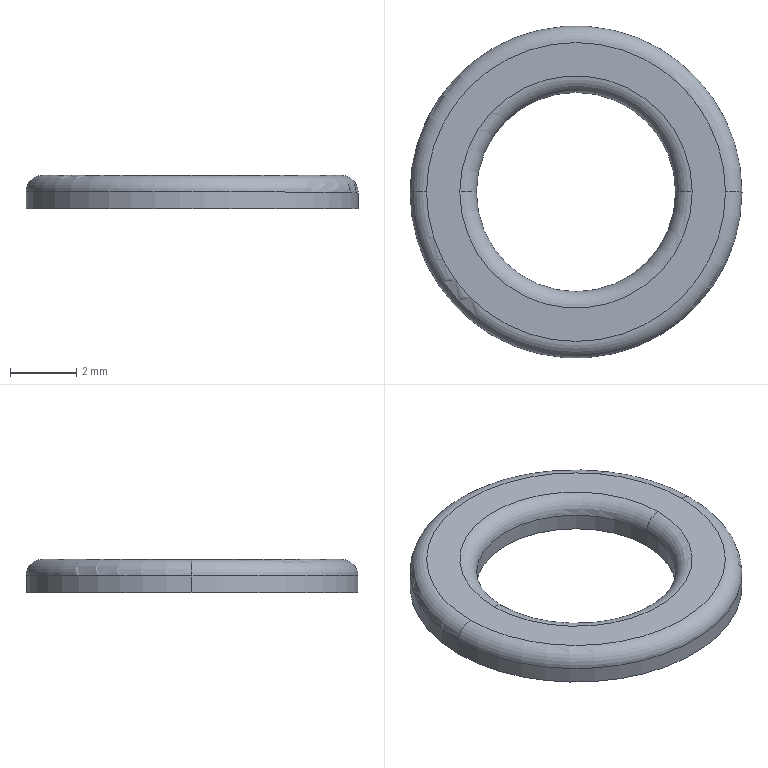Part | SolidWorks | features BaseBody 1 | 1 solid | 10 faces | box 10 x 10 x 1 mm | volume 47.569 mm3 | torus 4 | cylinder 4 | plane 2 | commonest cylinder face diameters 6 x2 10 x2
STEP:
#1=CARTESIAN_POINT('',(52.27,-94.624,-286.601));
#2=VERTEX_POINT('',#1);
#3=CARTESIAN_POINT('',(52.77,-94.624,-287.101));
#4=VERTEX_POINT('',#3);
#5=CARTESIAN_POINT('',(52.27,-94.624,-287.101));
#6=DIRECTION('',(0.,1.,0.));
#7=DIRECTION('',(0.,0.,1.));
#8=AXIS2_PLACEMENT_3D('',#5,#6,#7);
#9=CIRCLE('',#8,0.5);
#10=EDGE_CURVE('',#2,#4,#9,.T.);
#11=ORIENTED_EDGE('',*,*,#10,.T.);
#12=CARTESIAN_POINT('',(42.77,-94.624,-287.101));
#13=VERTEX_POINT('',#12);
#14=CARTESIAN_POINT('',(47.77,-94.624,-287.101));
#15=DIRECTION('',(0.,0.,-1.));
#16=DIRECTION('',(-0.9995,0.03075,0.));
#17=AXIS2_PLACEMENT_3D('',#14,#15,#16);
#18=CIRCLE('',#17,5.);
#19=EDGE_CURVE('',#13,#4,#18,.T.);
#20=ORIENTED_EDGE('',*,*,#19,.F.);
#21=CARTESIAN_POINT('',(43.27,-94.624,-286.601));
#22=VERTEX_POINT('',#21);
#23=CARTESIAN_POINT('',(43.27,-94.624,-287.101));
#24=DIRECTION('',(0.,-1.,0.));
#25=DIRECTION('',(0.,0.,1.));
#26=AXIS2_PLACEMENT_3D('',#23,#24,#25);
#27=CIRCLE('',#26,0.5);
#28=EDGE_CURVE('',#22,#13,#27,.T.);
#29=ORIENTED_EDGE('',*,*,#28,.F.);
#30=CARTESIAN_POINT('',(47.77,-94.624,-286.601));
#31=DIRECTION('',(0.,0.,1.));
#32=DIRECTION('',(-0.9995,0.03075,0.));
#33=AXIS2_PLACEMENT_3D('',#30,#31,#32);
#34=CIRCLE('',#33,4.5);
#35=EDGE_CURVE('',#2,#22,#34,.T.);
#36=ORIENTED_EDGE('',*,*,#35,.F.);
#37=EDGE_LOOP('',(#11,#20,#29,#36));
#38=FACE_OUTER_BOUND('',#37,.T.);
#39=CARTESIAN_POINT('',(47.77,-94.624,-287.101));
#40=DIRECTION('',(0.,0.,1.));
#41=DIRECTION('',(0.9995,-0.03075,0.));
#42=AXIS2_PLACEMENT_3D('',#39,#40,#41);
#43=TOROIDAL_SURFACE('',#42,4.5,0.5);
#44=ADVANCED_FACE('',(#38),#43,.T.);
#45=CARTESIAN_POINT('',(51.27,-94.624,-286.601));
#46=VERTEX_POINT('',#45);
#47=CARTESIAN_POINT('',(44.27,-94.624,-286.601));
#48=VERTEX_POINT('',#47);
#49=CARTESIAN_POINT('',(47.77,-94.624,-286.601));
#50=DIRECTION('',(0.,0.,1.));
#51=DIRECTION('',(0.9974,0.07275,0.));
#52=AXIS2_PLACEMENT_3D('',#49,#50,#51);
#53=CIRCLE('',#52,3.5);
#54=EDGE_CURVE('',#46,#48,#53,.T.);
#55=ORIENTED_EDGE('',*,*,#54,.F.);
#56=CARTESIAN_POINT('',(47.77,-94.624,-286.601));
#57=DIRECTION('',(0.,0.,1.));
#58=DIRECTION('',(-0.9974,-0.07275,0.));
#59=AXIS2_PLACEMENT_3D('',#56,#57,#58);
#60=CIRCLE('',#59,3.5);
#61=EDGE_CURVE('',#48,#46,#60,.T.);
#62=ORIENTED_EDGE('',*,*,#61,.F.);
#63=EDGE_LOOP('',(#55,#62));
#64=FACE_BOUND('',#63,.T.);
#65=CARTESIAN_POINT('',(47.77,-94.624,-286.601));
#66=DIRECTION('',(0.,0.,-1.));
#67=DIRECTION('',(0.9995,-0.03075,0.));
#68=AXIS2_PLACEMENT_3D('',#65,#66,#67);
#69=CIRCLE('',#68,4.5);
#70=EDGE_CURVE('',#2,#22,#69,.T.);
#71=ORIENTED_EDGE('',*,*,#70,.F.);
#72=ORIENTED_EDGE('',*,*,#35,.T.);
#73=EDGE_LOOP('',(#71,#72));
#74=FACE_OUTER_BOUND('',#73,.T.);
#75=CARTESIAN_POINT('',(-0.06299,0.3763,-286.601));
#76=DIRECTION('',(0.,0.,1.));
#77=DIRECTION('',(1.,0.,0.));
#78=AXIS2_PLACEMENT_3D('',#75,#76,#77);
#79=PLANE('',#78);
#80=ADVANCED_FACE('',(#64,#74),#79,.T.);
#81=ORIENTED_EDGE('',*,*,#28,.T.);
#82=CARTESIAN_POINT('',(47.77,-94.624,-287.101));
#83=DIRECTION('',(0.,0.,-1.));
#84=DIRECTION('',(0.9995,-0.03075,0.));
#85=AXIS2_PLACEMENT_3D('',#82,#83,#84);
#86=CIRCLE('',#85,5.);
#87=EDGE_CURVE('',#4,#13,#86,.T.);
#88=ORIENTED_EDGE('',*,*,#87,.F.);
#89=ORIENTED_EDGE('',*,*,#10,.F.);
#90=ORIENTED_EDGE('',*,*,#70,.T.);
#91=EDGE_LOOP('',(#81,#88,#89,#90));
#92=FACE_OUTER_BOUND('',#91,.T.);
#93=CARTESIAN_POINT('',(47.77,-94.624,-287.101));
#94=DIRECTION('',(0.,0.,1.));
#95=DIRECTION('',(-0.9995,0.03075,0.));
#96=AXIS2_PLACEMENT_3D('',#93,#94,#95);
#97=TOROIDAL_SURFACE('',#96,4.5,0.5);
#98=ADVANCED_FACE('',(#92),#97,.T.);
#99=CARTESIAN_POINT('',(42.77,-94.624,-287.601));
#100=VERTEX_POINT('',#99);
#101=CARTESIAN_POINT('',(42.77,-94.624,-287.601));
#102=DIRECTION('',(0.,0.,1.));
#103=VECTOR('',#102,1000.);
#104=LINE('',#101,#103);
#105=EDGE_CURVE('',#100,#13,#104,.T.);
#106=ORIENTED_EDGE('',*,*,#105,.F.);
#107=CARTESIAN_POINT('',(52.77,-94.624,-287.601));
#108=VERTEX_POINT('',#107);
#109=CARTESIAN_POINT('',(47.77,-94.624,-287.601));
#110=DIRECTION('',(0.,0.,1.));
#111=DIRECTION('',(-1.,0.,0.));
#112=AXIS2_PLACEMENT_3D('',#109,#110,#111);
#113=CIRCLE('',#112,5.);
#114=EDGE_CURVE('',#100,#108,#113,.T.);
#115=ORIENTED_EDGE('',*,*,#114,.T.);
#116=CARTESIAN_POINT('',(52.77,-94.624,-287.601));
#117=DIRECTION('',(0.,0.,1.));
#118=VECTOR('',#117,1000.);
#119=LINE('',#116,#118);
#120=EDGE_CURVE('',#108,#4,#119,.T.);
#121=ORIENTED_EDGE('',*,*,#120,.T.);
#122=ORIENTED_EDGE('',*,*,#87,.T.);
#123=EDGE_LOOP('',(#106,#115,#121,#122));
#124=FACE_OUTER_BOUND('',#123,.T.);
#125=CARTESIAN_POINT('',(47.77,-94.624,-287.601));
#126=DIRECTION('',(0.,0.,1.));
#127=DIRECTION('',(-1.,0.,0.));
#128=AXIS2_PLACEMENT_3D('',#125,#126,#127);
#129=CYLINDRICAL_SURFACE('',#128,5.);
#130=ADVANCED_FACE('',(#124),#129,.T.);
#131=ORIENTED_EDGE('',*,*,#120,.F.);
#132=CARTESIAN_POINT('',(47.77,-94.624,-287.601));
#133=DIRECTION('',(0.,0.,1.));
#134=DIRECTION('',(1.,0.,0.));
#135=AXIS2_PLACEMENT_3D('',#132,#133,#134);
#136=CIRCLE('',#135,5.);
#137=EDGE_CURVE('',#108,#100,#136,.T.);
#138=ORIENTED_EDGE('',*,*,#137,.T.);
#139=ORIENTED_EDGE('',*,*,#105,.T.);
#140=ORIENTED_EDGE('',*,*,#19,.T.);
#141=EDGE_LOOP('',(#131,#138,#139,#140));
#142=FACE_OUTER_BOUND('',#141,.T.);
#143=CARTESIAN_POINT('',(47.77,-94.624,-287.601));
#144=DIRECTION('',(0.,0.,1.));
#145=DIRECTION('',(-1.,0.,0.));
#146=AXIS2_PLACEMENT_3D('',#143,#144,#145);
#147=CYLINDRICAL_SURFACE('',#146,5.);
#148=ADVANCED_FACE('',(#142),#147,.T.);
#149=CARTESIAN_POINT('',(50.77,-94.624,-287.601));
#150=VERTEX_POINT('',#149);
#151=CARTESIAN_POINT('',(44.77,-94.624,-287.601));
#152=VERTEX_POINT('',#151);
#153=CARTESIAN_POINT('',(47.77,-94.624,-287.601));
#154=DIRECTION('',(0.,0.,-1.));
#155=DIRECTION('',(1.,0.,0.));
#156=AXIS2_PLACEMENT_3D('',#153,#154,#155);
#157=CIRCLE('',#156,3.);
#158=EDGE_CURVE('',#150,#152,#157,.T.);
#159=ORIENTED_EDGE('',*,*,#158,.F.);
#160=CARTESIAN_POINT('',(47.77,-94.624,-287.601));
#161=DIRECTION('',(0.,0.,-1.));
#162=DIRECTION('',(-1.,0.,0.));
#163=AXIS2_PLACEMENT_3D('',#160,#161,#162);
#164=CIRCLE('',#163,3.);
#165=EDGE_CURVE('',#152,#150,#164,.T.);
#166=ORIENTED_EDGE('',*,*,#165,.F.);
#167=EDGE_LOOP('',(#159,#166));
#168=FACE_BOUND('',#167,.T.);
#169=ORIENTED_EDGE('',*,*,#137,.F.);
#170=ORIENTED_EDGE('',*,*,#114,.F.);
#171=EDGE_LOOP('',(#169,#170));
#172=FACE_OUTER_BOUND('',#171,.T.);
#173=CARTESIAN_POINT('',(-0.06299,0.3763,-287.601));
#174=DIRECTION('',(0.,0.,1.));
#175=DIRECTION('',(1.,0.,0.));
#176=AXIS2_PLACEMENT_3D('',#173,#174,#175);
#177=PLANE('',#176);
#178=ADVANCED_FACE('',(#168,#172),#177,.F.);
#179=CARTESIAN_POINT('',(44.77,-94.624,-287.101));
#180=VERTEX_POINT('',#179);
#181=CARTESIAN_POINT('',(44.77,-94.624,-287.601));
#182=DIRECTION('',(0.,0.,1.));
#183=VECTOR('',#182,1000.);
#184=LINE('',#181,#183);
#185=EDGE_CURVE('',#152,#180,#184,.T.);
#186=ORIENTED_EDGE('',*,*,#185,.F.);
#187=ORIENTED_EDGE('',*,*,#165,.T.);
#188=CARTESIAN_POINT('',(50.77,-94.624,-287.101));
#189=VERTEX_POINT('',#188);
#190=CARTESIAN_POINT('',(50.77,-94.624,-287.601));
#191=DIRECTION('',(0.,0.,1.));
#192=VECTOR('',#191,1000.);
#193=LINE('',#190,#192);
#194=EDGE_CURVE('',#150,#189,#193,.T.);
#195=ORIENTED_EDGE('',*,*,#194,.T.);
#196=CARTESIAN_POINT('',(47.77,-94.624,-287.101));
#197=DIRECTION('',(0.,0.,1.));
#198=DIRECTION('',(1.,0.,0.));
#199=AXIS2_PLACEMENT_3D('',#196,#197,#198);
#200=CIRCLE('',#199,3.);
#201=EDGE_CURVE('',#189,#180,#200,.T.);
#202=ORIENTED_EDGE('',*,*,#201,.T.);
#203=EDGE_LOOP('',(#186,#187,#195,#202));
#204=FACE_OUTER_BOUND('',#203,.T.);
#205=CARTESIAN_POINT('',(47.77,-94.624,-287.601));
#206=DIRECTION('',(0.,0.,1.));
#207=DIRECTION('',(-1.,0.,0.));
#208=AXIS2_PLACEMENT_3D('',#205,#206,#207);
#209=CYLINDRICAL_SURFACE('',#208,3.);
#210=ADVANCED_FACE('',(#204),#209,.F.);
#211=CARTESIAN_POINT('',(44.27,-94.624,-287.101));
#212=DIRECTION('',(0.,1.,0.));
#213=DIRECTION('',(0.,0.,1.));
#214=AXIS2_PLACEMENT_3D('',#211,#212,#213);
#215=CIRCLE('',#214,0.5);
#216=EDGE_CURVE('',#48,#180,#215,.T.);
#217=ORIENTED_EDGE('',*,*,#216,.T.);
#218=ORIENTED_EDGE('',*,*,#201,.F.);
#219=CARTESIAN_POINT('',(51.27,-94.624,-287.101));
#220=DIRECTION('',(0.,-1.,0.));
#221=DIRECTION('',(0.,0.,1.));
#222=AXIS2_PLACEMENT_3D('',#219,#220,#221);
#223=CIRCLE('',#222,0.5);
#224=EDGE_CURVE('',#46,#189,#223,.T.);
#225=ORIENTED_EDGE('',*,*,#224,.F.);
#226=ORIENTED_EDGE('',*,*,#54,.T.);
#227=EDGE_LOOP('',(#217,#218,#225,#226));
#228=FACE_OUTER_BOUND('',#227,.T.);
#229=CARTESIAN_POINT('',(47.77,-94.624,-287.101));
#230=DIRECTION('',(0.,0.,1.));
#231=DIRECTION('',(-0.9974,-0.07275,0.));
#232=AXIS2_PLACEMENT_3D('',#229,#230,#231);
#233=TOROIDAL_SURFACE('',#232,3.5,0.5);
#234=ADVANCED_FACE('',(#228),#233,.T.);
#235=ORIENTED_EDGE('',*,*,#224,.T.);
#236=CARTESIAN_POINT('',(47.77,-94.624,-287.101));
#237=DIRECTION('',(0.,0.,1.));
#238=DIRECTION('',(-0.9974,-0.07275,0.));
#239=AXIS2_PLACEMENT_3D('',#236,#237,#238);
#240=CIRCLE('',#239,3.);
#241=EDGE_CURVE('',#180,#189,#240,.T.);
#242=ORIENTED_EDGE('',*,*,#241,.F.);
#243=ORIENTED_EDGE('',*,*,#216,.F.);
#244=ORIENTED_EDGE('',*,*,#61,.T.);
#245=EDGE_LOOP('',(#235,#242,#243,#244));
#246=FACE_OUTER_BOUND('',#245,.T.);
#247=CARTESIAN_POINT('',(47.77,-94.624,-287.101));
#248=DIRECTION('',(0.,0.,1.));
#249=DIRECTION('',(0.9974,0.07275,0.));
#250=AXIS2_PLACEMENT_3D('',#247,#248,#249);
#251=TOROIDAL_SURFACE('',#250,3.5,0.5);
#252=ADVANCED_FACE('',(#246),#251,.T.);
#253=ORIENTED_EDGE('',*,*,#194,.F.);
#254=ORIENTED_EDGE('',*,*,#158,.T.);
#255=ORIENTED_EDGE('',*,*,#185,.T.);
#256=ORIENTED_EDGE('',*,*,#241,.T.);
#257=EDGE_LOOP('',(#253,#254,#255,#256));
#258=FACE_OUTER_BOUND('',#257,.T.);
#259=CARTESIAN_POINT('',(47.77,-94.624,-287.601));
#260=DIRECTION('',(0.,0.,1.));
#261=DIRECTION('',(-1.,0.,0.));
#262=AXIS2_PLACEMENT_3D('',#259,#260,#261);
#263=CYLINDRICAL_SURFACE('',#262,3.);
#264=ADVANCED_FACE('',(#258),#263,.F.);
#265=CLOSED_SHELL('',(#44,#80,#98,#130,#148,#178,#210,#234,#252,#264));
#266=MANIFOLD_SOLID_BREP('',#265);
#267=CARTESIAN_POINT('',(0.,0.,0.));
#268=DIRECTION('',(0.,0.,1.));
#269=DIRECTION('',(1.,0.,0.));
#270=AXIS2_PLACEMENT_3D('',#267,#268,#269);
#271=(LENGTH_UNIT()NAMED_UNIT(*)SI_UNIT(.MILLI.,.METRE.));
#272=UNCERTAINTY_MEASURE_WITH_UNIT(LENGTH_MEASURE(0.00001),#271,'','');
#273=(NAMED_UNIT(*)PLANE_ANGLE_UNIT()SI_UNIT($,.RADIAN.));
#274=(NAMED_UNIT(*)SI_UNIT($,.STERADIAN.)SOLID_ANGLE_UNIT());
#275=(GEOMETRIC_REPRESENTATION_CONTEXT(3)GLOBAL_UNCERTAINTY_ASSIGNED_CONTEXT((#272))GLOBAL_UNIT_ASSIGNED_CONTEXT((#271,#273,#274))REPRESENTATION_CONTEXT('',''));
#276=ADVANCED_BREP_SHAPE_REPRESENTATION('',(#266,#270),#275);